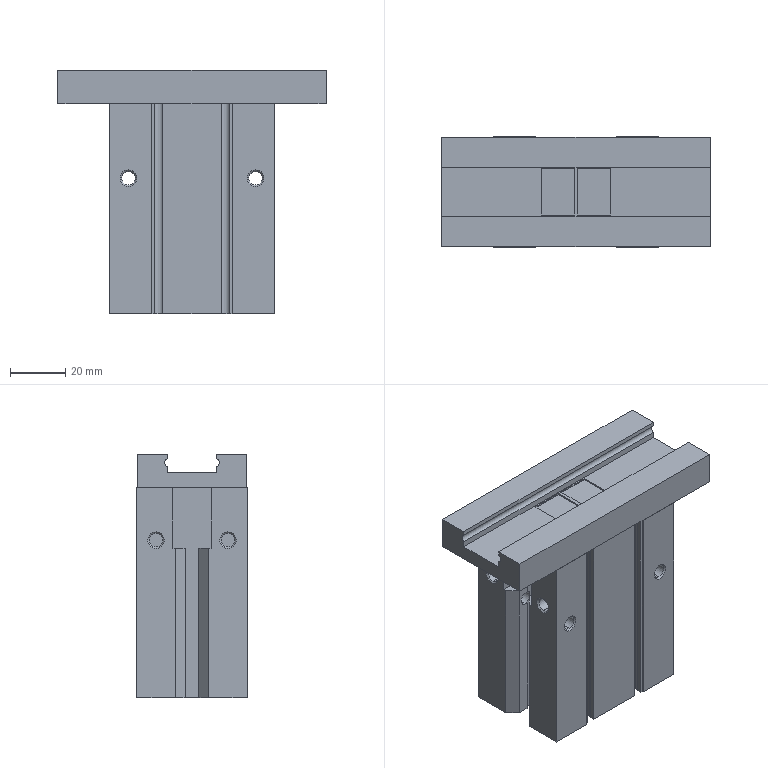Part | SolidWorks | features BaseBody 1 | 1 solid | 167 faces | box 97 x 40 x 88 mm | volume 188244 mm3 | plane 97 | cylinder 44 | cone 26 | commonest cylinder face diameters 4.917 x16 4 x12 5.1 x8 3.174 x2 4.134 x2 5 x2